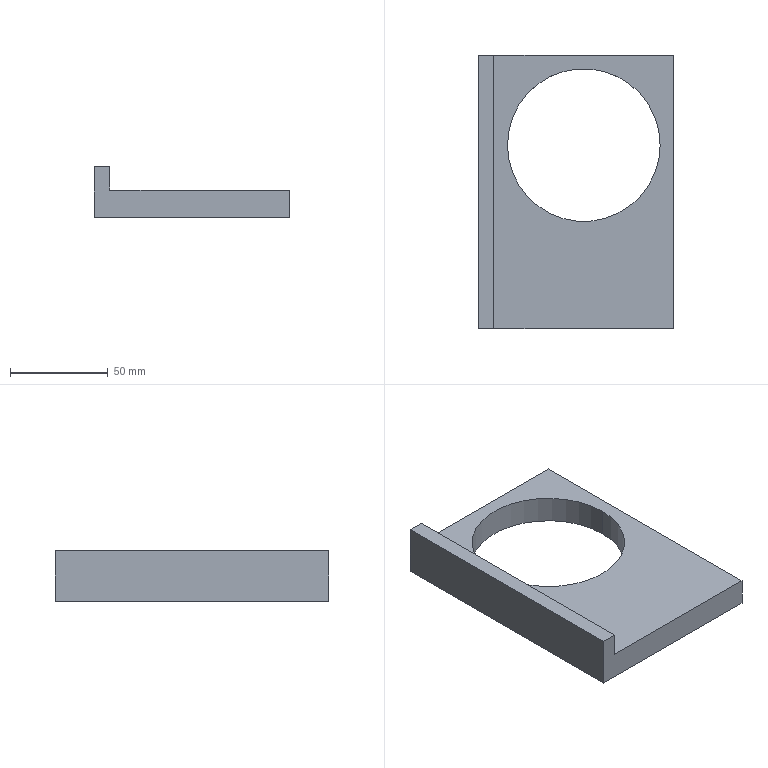Part | SolidWorks | features ICE 2, Extrusion 1 | 1 solid | 10 faces | box 100 x 140 x 26 mm | volume 142543 mm3 | plane 8 | cylinder 2 | commonest cylinder face diameters 78 x2
STEP:
#1=CARTESIAN_POINT('',(-35.,24.,0.));
#2=VERTEX_POINT('',#1);
#3=CARTESIAN_POINT('',(43.,24.,0.));
#4=VERTEX_POINT('',#3);
#5=CARTESIAN_POINT('',(4.,24.,0.));
#6=DIRECTION('',(0.,0.,1.));
#7=DIRECTION('',(-1.,0.,0.));
#8=AXIS2_PLACEMENT_3D('',#5,#6,#7);
#9=CIRCLE('',#8,39.);
#10=EDGE_CURVE('',#2,#4,#9,.T.);
#11=ORIENTED_EDGE('',*,*,#10,.F.);
#12=CARTESIAN_POINT('',(-35.,24.,14.));
#13=VERTEX_POINT('',#12);
#14=CARTESIAN_POINT('',(-35.,24.,-0.001));
#15=DIRECTION('',(0.,0.,1.));
#16=VECTOR('',#15,1000.);
#17=LINE('',#14,#16);
#18=EDGE_CURVE('',#2,#13,#17,.T.);
#19=ORIENTED_EDGE('',*,*,#18,.T.);
#20=CARTESIAN_POINT('',(43.,24.,14.));
#21=VERTEX_POINT('',#20);
#22=CARTESIAN_POINT('',(4.,24.,14.));
#23=DIRECTION('',(0.,0.,1.));
#24=DIRECTION('',(1.,0.,0.));
#25=AXIS2_PLACEMENT_3D('',#22,#23,#24);
#26=CIRCLE('',#25,39.);
#27=EDGE_CURVE('',#13,#21,#26,.T.);
#28=ORIENTED_EDGE('',*,*,#27,.T.);
#29=CARTESIAN_POINT('',(43.,24.,-0.001));
#30=DIRECTION('',(0.,0.,1.));
#31=VECTOR('',#30,1000.);
#32=LINE('',#29,#31);
#33=EDGE_CURVE('',#4,#21,#32,.T.);
#34=ORIENTED_EDGE('',*,*,#33,.F.);
#35=EDGE_LOOP('',(#11,#19,#28,#34));
#36=FACE_OUTER_BOUND('',#35,.T.);
#37=CARTESIAN_POINT('',(4.,24.,-0.001));
#38=DIRECTION('',(0.,0.,1.));
#39=DIRECTION('',(1.,0.,0.));
#40=AXIS2_PLACEMENT_3D('',#37,#38,#39);
#41=CYLINDRICAL_SURFACE('',#40,39.);
#42=ADVANCED_FACE('',(#36),#41,.F.);
#43=CARTESIAN_POINT('',(4.,24.,14.));
#44=DIRECTION('',(0.,0.,1.));
#45=DIRECTION('',(1.,0.,0.));
#46=AXIS2_PLACEMENT_3D('',#43,#44,#45);
#47=CIRCLE('',#46,39.);
#48=EDGE_CURVE('',#21,#13,#47,.T.);
#49=ORIENTED_EDGE('',*,*,#48,.F.);
#50=ORIENTED_EDGE('',*,*,#27,.F.);
#51=EDGE_LOOP('',(#49,#50));
#52=FACE_BOUND('',#51,.T.);
#53=CARTESIAN_POINT('',(-42.,-70.,14.));
#54=VERTEX_POINT('',#53);
#55=CARTESIAN_POINT('',(-42.,70.,14.));
#56=VERTEX_POINT('',#55);
#57=CARTESIAN_POINT('',(-42.,70.,14.));
#58=DIRECTION('',(0.,1.,0.));
#59=VECTOR('',#58,1000.);
#60=LINE('',#57,#59);
#61=EDGE_CURVE('',#54,#56,#60,.T.);
#62=ORIENTED_EDGE('',*,*,#61,.F.);
#63=CARTESIAN_POINT('',(50.,-70.,14.));
#64=VERTEX_POINT('',#63);
#65=CARTESIAN_POINT('',(-50.,-70.,14.));
#66=DIRECTION('',(1.,0.,0.));
#67=VECTOR('',#66,1000.);
#68=LINE('',#65,#67);
#69=EDGE_CURVE('',#54,#64,#68,.T.);
#70=ORIENTED_EDGE('',*,*,#69,.T.);
#71=CARTESIAN_POINT('',(50.,70.,14.));
#72=VERTEX_POINT('',#71);
#73=CARTESIAN_POINT('',(50.,-70.,14.));
#74=DIRECTION('',(0.,1.,0.));
#75=VECTOR('',#74,1000.);
#76=LINE('',#73,#75);
#77=EDGE_CURVE('',#64,#72,#76,.T.);
#78=ORIENTED_EDGE('',*,*,#77,.T.);
#79=CARTESIAN_POINT('',(-50.,70.,14.));
#80=DIRECTION('',(-1.,0.,0.));
#81=VECTOR('',#80,1000.);
#82=LINE('',#79,#81);
#83=EDGE_CURVE('',#72,#56,#82,.T.);
#84=ORIENTED_EDGE('',*,*,#83,.T.);
#85=EDGE_LOOP('',(#62,#70,#78,#84));
#86=FACE_OUTER_BOUND('',#85,.T.);
#87=CARTESIAN_POINT('',(0.,0.,14.));
#88=DIRECTION('',(0.,0.,-1.));
#89=DIRECTION('',(-1.,0.,0.));
#90=AXIS2_PLACEMENT_3D('',#87,#88,#89);
#91=PLANE('',#90);
#92=ADVANCED_FACE('',(#52,#86),#91,.F.);
#93=CARTESIAN_POINT('',(50.,-70.,0.));
#94=VERTEX_POINT('',#93);
#95=CARTESIAN_POINT('',(50.,70.,0.));
#96=VERTEX_POINT('',#95);
#97=CARTESIAN_POINT('',(50.,-70.,0.));
#98=DIRECTION('',(0.,1.,0.));
#99=VECTOR('',#98,1000.);
#100=LINE('',#97,#99);
#101=EDGE_CURVE('',#94,#96,#100,.T.);
#102=ORIENTED_EDGE('',*,*,#101,.T.);
#103=CARTESIAN_POINT('',(50.,70.,14.));
#104=DIRECTION('',(0.,0.,-1.));
#105=VECTOR('',#104,1000.);
#106=LINE('',#103,#105);
#107=EDGE_CURVE('',#72,#96,#106,.T.);
#108=ORIENTED_EDGE('',*,*,#107,.F.);
#109=ORIENTED_EDGE('',*,*,#77,.F.);
#110=CARTESIAN_POINT('',(50.,-70.,14.));
#111=DIRECTION('',(0.,0.,-1.));
#112=VECTOR('',#111,1000.);
#113=LINE('',#110,#112);
#114=EDGE_CURVE('',#64,#94,#113,.T.);
#115=ORIENTED_EDGE('',*,*,#114,.T.);
#116=EDGE_LOOP('',(#102,#108,#109,#115));
#117=FACE_OUTER_BOUND('',#116,.T.);
#118=CARTESIAN_POINT('',(50.,-70.,14.));
#119=DIRECTION('',(-1.,0.,0.));
#120=DIRECTION('',(0.,0.,1.));
#121=AXIS2_PLACEMENT_3D('',#118,#119,#120);
#122=PLANE('',#121);
#123=ADVANCED_FACE('',(#117),#122,.F.);
#124=CARTESIAN_POINT('',(-50.,70.,0.));
#125=VERTEX_POINT('',#124);
#126=CARTESIAN_POINT('',(-50.,70.,0.));
#127=DIRECTION('',(-1.,0.,0.));
#128=VECTOR('',#127,1000.);
#129=LINE('',#126,#128);
#130=EDGE_CURVE('',#96,#125,#129,.T.);
#131=ORIENTED_EDGE('',*,*,#130,.T.);
#132=CARTESIAN_POINT('',(-50.,70.,26.));
#133=VERTEX_POINT('',#132);
#134=CARTESIAN_POINT('',(-50.,70.,14.));
#135=DIRECTION('',(0.,0.,-1.));
#136=VECTOR('',#135,1000.);
#137=LINE('',#134,#136);
#138=EDGE_CURVE('',#133,#125,#137,.T.);
#139=ORIENTED_EDGE('',*,*,#138,.F.);
#140=CARTESIAN_POINT('',(-42.,70.,26.));
#141=VERTEX_POINT('',#140);
#142=CARTESIAN_POINT('',(-50.,70.,26.));
#143=DIRECTION('',(-1.,0.,0.));
#144=VECTOR('',#143,1000.);
#145=LINE('',#142,#144);
#146=EDGE_CURVE('',#141,#133,#145,.T.);
#147=ORIENTED_EDGE('',*,*,#146,.F.);
#148=CARTESIAN_POINT('',(-42.,70.,26.));
#149=DIRECTION('',(0.,0.,-1.));
#150=VECTOR('',#149,1000.);
#151=LINE('',#148,#150);
#152=EDGE_CURVE('',#141,#56,#151,.T.);
#153=ORIENTED_EDGE('',*,*,#152,.T.);
#154=ORIENTED_EDGE('',*,*,#83,.F.);
#155=ORIENTED_EDGE('',*,*,#107,.T.);
#156=EDGE_LOOP('',(#131,#139,#147,#153,#154,#155));
#157=FACE_OUTER_BOUND('',#156,.T.);
#158=CARTESIAN_POINT('',(-50.,70.,14.));
#159=DIRECTION('',(0.,-1.,0.));
#160=DIRECTION('',(0.,0.,-1.));
#161=AXIS2_PLACEMENT_3D('',#158,#159,#160);
#162=PLANE('',#161);
#163=ADVANCED_FACE('',(#157),#162,.F.);
#164=CARTESIAN_POINT('',(-50.,-70.,0.));
#165=VERTEX_POINT('',#164);
#166=CARTESIAN_POINT('',(-50.,-70.,0.));
#167=DIRECTION('',(0.,-1.,0.));
#168=VECTOR('',#167,1000.);
#169=LINE('',#166,#168);
#170=EDGE_CURVE('',#125,#165,#169,.T.);
#171=ORIENTED_EDGE('',*,*,#170,.T.);
#172=CARTESIAN_POINT('',(-50.,-70.,26.));
#173=VERTEX_POINT('',#172);
#174=CARTESIAN_POINT('',(-50.,-70.,14.));
#175=DIRECTION('',(0.,0.,-1.));
#176=VECTOR('',#175,1000.);
#177=LINE('',#174,#176);
#178=EDGE_CURVE('',#173,#165,#177,.T.);
#179=ORIENTED_EDGE('',*,*,#178,.F.);
#180=CARTESIAN_POINT('',(-50.,70.,26.));
#181=DIRECTION('',(0.,-1.,0.));
#182=VECTOR('',#181,1000.);
#183=LINE('',#180,#182);
#184=EDGE_CURVE('',#133,#173,#183,.T.);
#185=ORIENTED_EDGE('',*,*,#184,.F.);
#186=ORIENTED_EDGE('',*,*,#138,.T.);
#187=EDGE_LOOP('',(#171,#179,#185,#186));
#188=FACE_OUTER_BOUND('',#187,.T.);
#189=CARTESIAN_POINT('',(-50.,-70.,14.));
#190=DIRECTION('',(1.,0.,0.));
#191=DIRECTION('',(0.,0.,-1.));
#192=AXIS2_PLACEMENT_3D('',#189,#190,#191);
#193=PLANE('',#192);
#194=ADVANCED_FACE('',(#188),#193,.F.);
#195=CARTESIAN_POINT('',(-50.,-70.,0.));
#196=DIRECTION('',(1.,0.,0.));
#197=VECTOR('',#196,1000.);
#198=LINE('',#195,#197);
#199=EDGE_CURVE('',#165,#94,#198,.T.);
#200=ORIENTED_EDGE('',*,*,#199,.T.);
#201=ORIENTED_EDGE('',*,*,#114,.F.);
#202=ORIENTED_EDGE('',*,*,#69,.F.);
#203=CARTESIAN_POINT('',(-42.,-70.,26.));
#204=VERTEX_POINT('',#203);
#205=CARTESIAN_POINT('',(-42.,-70.,26.));
#206=DIRECTION('',(0.,0.,-1.));
#207=VECTOR('',#206,1000.);
#208=LINE('',#205,#207);
#209=EDGE_CURVE('',#204,#54,#208,.T.);
#210=ORIENTED_EDGE('',*,*,#209,.F.);
#211=CARTESIAN_POINT('',(-50.,-70.,26.));
#212=DIRECTION('',(1.,0.,0.));
#213=VECTOR('',#212,1000.);
#214=LINE('',#211,#213);
#215=EDGE_CURVE('',#173,#204,#214,.T.);
#216=ORIENTED_EDGE('',*,*,#215,.F.);
#217=ORIENTED_EDGE('',*,*,#178,.T.);
#218=EDGE_LOOP('',(#200,#201,#202,#210,#216,#217));
#219=FACE_OUTER_BOUND('',#218,.T.);
#220=CARTESIAN_POINT('',(-50.,-70.,14.));
#221=DIRECTION('',(0.,1.,0.));
#222=DIRECTION('',(0.,0.,1.));
#223=AXIS2_PLACEMENT_3D('',#220,#221,#222);
#224=PLANE('',#223);
#225=ADVANCED_FACE('',(#219),#224,.F.);
#226=CARTESIAN_POINT('',(4.,24.,0.));
#227=DIRECTION('',(0.,0.,1.));
#228=DIRECTION('',(-1.,0.,0.));
#229=AXIS2_PLACEMENT_3D('',#226,#227,#228);
#230=CIRCLE('',#229,39.);
#231=EDGE_CURVE('',#4,#2,#230,.T.);
#232=ORIENTED_EDGE('',*,*,#231,.T.);
#233=ORIENTED_EDGE('',*,*,#10,.T.);
#234=EDGE_LOOP('',(#232,#233));
#235=FACE_BOUND('',#234,.T.);
#236=ORIENTED_EDGE('',*,*,#101,.F.);
#237=ORIENTED_EDGE('',*,*,#199,.F.);
#238=ORIENTED_EDGE('',*,*,#170,.F.);
#239=ORIENTED_EDGE('',*,*,#130,.F.);
#240=EDGE_LOOP('',(#236,#237,#238,#239));
#241=FACE_OUTER_BOUND('',#240,.T.);
#242=CARTESIAN_POINT('',(0.,0.,0.));
#243=DIRECTION('',(0.,0.,-1.));
#244=DIRECTION('',(-1.,0.,0.));
#245=AXIS2_PLACEMENT_3D('',#242,#243,#244);
#246=PLANE('',#245);
#247=ADVANCED_FACE('',(#235,#241),#246,.T.);
#248=ORIENTED_EDGE('',*,*,#18,.F.);
#249=ORIENTED_EDGE('',*,*,#231,.F.);
#250=ORIENTED_EDGE('',*,*,#33,.T.);
#251=ORIENTED_EDGE('',*,*,#48,.T.);
#252=EDGE_LOOP('',(#248,#249,#250,#251));
#253=FACE_OUTER_BOUND('',#252,.T.);
#254=CARTESIAN_POINT('',(4.,24.,-0.001));
#255=DIRECTION('',(0.,0.,1.));
#256=DIRECTION('',(1.,0.,0.));
#257=AXIS2_PLACEMENT_3D('',#254,#255,#256);
#258=CYLINDRICAL_SURFACE('',#257,39.);
#259=ADVANCED_FACE('',(#253),#258,.F.);
#260=ORIENTED_EDGE('',*,*,#61,.T.);
#261=ORIENTED_EDGE('',*,*,#152,.F.);
#262=CARTESIAN_POINT('',(-42.,70.,26.));
#263=DIRECTION('',(0.,1.,0.));
#264=VECTOR('',#263,1000.);
#265=LINE('',#262,#264);
#266=EDGE_CURVE('',#204,#141,#265,.T.);
#267=ORIENTED_EDGE('',*,*,#266,.F.);
#268=ORIENTED_EDGE('',*,*,#209,.T.);
#269=EDGE_LOOP('',(#260,#261,#267,#268));
#270=FACE_OUTER_BOUND('',#269,.T.);
#271=CARTESIAN_POINT('',(-42.,70.,26.));
#272=DIRECTION('',(-1.,0.,0.));
#273=DIRECTION('',(0.,-1.,0.));
#274=AXIS2_PLACEMENT_3D('',#271,#272,#273);
#275=PLANE('',#274);
#276=ADVANCED_FACE('',(#270),#275,.F.);
#277=ORIENTED_EDGE('',*,*,#184,.T.);
#278=ORIENTED_EDGE('',*,*,#215,.T.);
#279=ORIENTED_EDGE('',*,*,#266,.T.);
#280=ORIENTED_EDGE('',*,*,#146,.T.);
#281=EDGE_LOOP('',(#277,#278,#279,#280));
#282=FACE_OUTER_BOUND('',#281,.T.);
#283=CARTESIAN_POINT('',(0.,0.,26.));
#284=DIRECTION('',(0.,0.,1.));
#285=DIRECTION('',(1.,0.,0.));
#286=AXIS2_PLACEMENT_3D('',#283,#284,#285);
#287=PLANE('',#286);
#288=ADVANCED_FACE('',(#282),#287,.T.);
#289=CLOSED_SHELL('',(#42,#92,#123,#163,#194,#225,#247,#259,#276,#288));
#290=MANIFOLD_SOLID_BREP('',#289);
#291=CARTESIAN_POINT('',(0.,0.,0.));
#292=DIRECTION('',(0.,0.,1.));
#293=DIRECTION('',(1.,0.,0.));
#294=AXIS2_PLACEMENT_3D('',#291,#292,#293);
#295=(LENGTH_UNIT()NAMED_UNIT(*)SI_UNIT(.MILLI.,.METRE.));
#296=UNCERTAINTY_MEASURE_WITH_UNIT(LENGTH_MEASURE(0.00001),#295,'','');
#297=(NAMED_UNIT(*)PLANE_ANGLE_UNIT()SI_UNIT($,.RADIAN.));
#298=(NAMED_UNIT(*)SI_UNIT($,.STERADIAN.)SOLID_ANGLE_UNIT());
#299=(GEOMETRIC_REPRESENTATION_CONTEXT(3)GLOBAL_UNCERTAINTY_ASSIGNED_CONTEXT((#296))GLOBAL_UNIT_ASSIGNED_CONTEXT((#295,#297,#298))REPRESENTATION_CONTEXT('',''));
#300=ADVANCED_BREP_SHAPE_REPRESENTATION('',(#290,#294),#299);